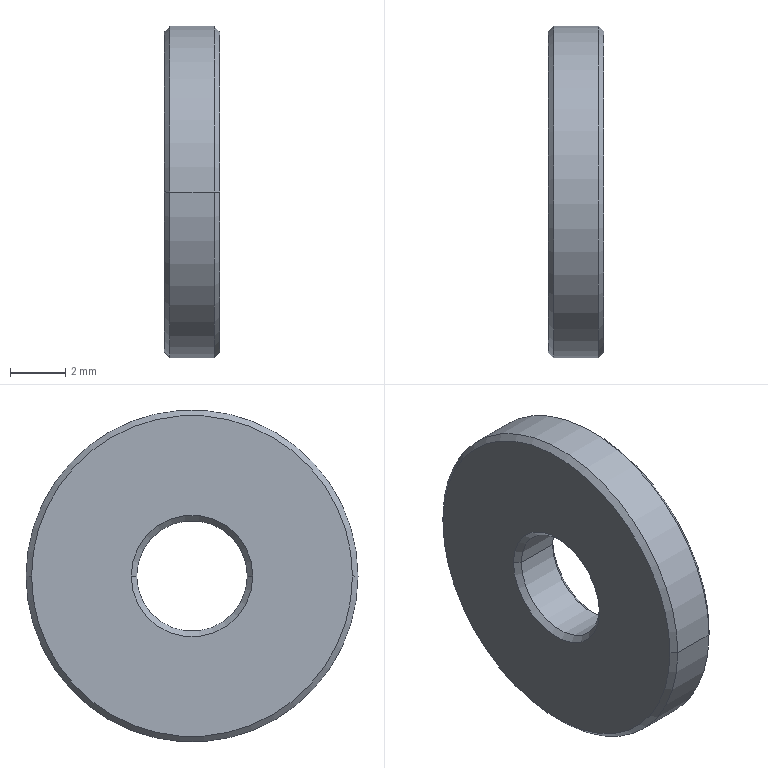Part | STEP file | wasmh12_4_2_2_03 | 1 solid | 14 faces | box 2 x 12 x 12 mm | volume 199.051 mm3 | cone 8 | cylinder 4 | plane 2 | commonest cylinder face diameters 4 x2 12 x2
STEP:
#1=CARTESIAN_POINT('',(0.,0.,0.));
#2=DIRECTION('',(0.,0.,1.));
#3=DIRECTION('',(1.,0.,0.));
#4=AXIS2_PLACEMENT_3D('',#1,#2,#3);
#5=CARTESIAN_POINT('',(0.2,-2.,0.));
#6=VERTEX_POINT('',#5);
#7=CARTESIAN_POINT('',(0.,-2.2,0.));
#8=VERTEX_POINT('',#7);
#9=CARTESIAN_POINT('',(0.,-2.2,0.));
#10=DIRECTION('',(-0.7071,-0.7071,0.));
#11=VECTOR('',#10,1.);
#12=LINE('',#9,#11);
#13=CARTESIAN_POINT('',(0.,0.,0.));
#14=DIRECTION('',(-1.,0.,0.));
#15=DIRECTION('',(0.,-1.,0.));
#16=AXIS2_PLACEMENT_3D('',#13,#14,#15);
#17=CONICAL_SURFACE('',#16,2.2,0.7854);
#18=CARTESIAN_POINT('',(6.283,0.));
#19=DIRECTION('',(0.,1.));
#20=VECTOR('',#19,1.);
#21=LINE('',#18,#20);
#22=(GEOMETRIC_REPRESENTATION_CONTEXT(2)PARAMETRIC_REPRESENTATION_CONTEXT()REPRESENTATION_CONTEXT('',''));
#23=DEFINITIONAL_REPRESENTATION('',(#21),#22);
#24=PCURVE('',#17,#23);
#25=CARTESIAN_POINT('',(0.,0.,0.));
#26=DIRECTION('',(-1.,0.,0.));
#27=DIRECTION('',(0.,-1.,0.));
#28=AXIS2_PLACEMENT_3D('',#25,#26,#27);
#29=CONICAL_SURFACE('',#28,2.2,0.7854);
#30=CARTESIAN_POINT('',(0.,0.));
#31=DIRECTION('',(0.,1.));
#32=VECTOR('',#31,1.);
#33=LINE('',#30,#32);
#34=(GEOMETRIC_REPRESENTATION_CONTEXT(2)PARAMETRIC_REPRESENTATION_CONTEXT()REPRESENTATION_CONTEXT('',''));
#35=DEFINITIONAL_REPRESENTATION('',(#33),#34);
#36=PCURVE('',#29,#35);
#37=SURFACE_CURVE('',#12,(#24,#36),.PCURVE_S1.);
#38=EDGE_CURVE('',#6,#8,#37,.T.);
#39=ORIENTED_EDGE('',*,*,#38,.T.);
#40=CARTESIAN_POINT('',(0.,2.2,0.));
#41=VERTEX_POINT('',#40);
#42=CARTESIAN_POINT('',(0.,0.,0.));
#43=DIRECTION('',(1.,0.,0.));
#44=DIRECTION('',(0.,-1.,0.));
#45=AXIS2_PLACEMENT_3D('',#42,#43,#44);
#46=CIRCLE('',#45,2.2);
#47=CARTESIAN_POINT('',(6.283,0.));
#48=DIRECTION('',(-1.,0.));
#49=VECTOR('',#48,1.);
#50=LINE('',#47,#49);
#51=(GEOMETRIC_REPRESENTATION_CONTEXT(2)PARAMETRIC_REPRESENTATION_CONTEXT()REPRESENTATION_CONTEXT('',''));
#52=DEFINITIONAL_REPRESENTATION('',(#50),#51);
#53=PCURVE('',#17,#52);
#54=CARTESIAN_POINT('',(0.,-4.,0.));
#55=DIRECTION('',(-1.,0.,0.));
#56=DIRECTION('',(0.,-1.,0.));
#57=AXIS2_PLACEMENT_3D('',#54,#55,#56);
#58=PLANE('',#57);
#59=CARTESIAN_POINT('',(-1.8,0.));
#60=CARTESIAN_POINT('',(-1.8,-3.811));
#61=CARTESIAN_POINT('',(-5.1,-1.905));
#62=CARTESIAN_POINT('',(-8.4,0.));
#63=CARTESIAN_POINT('',(-5.1,1.905));
#64=CARTESIAN_POINT('',(-1.8,3.811));
#65=CARTESIAN_POINT('',(-1.8,0.));
#66=(BOUNDED_CURVE()B_SPLINE_CURVE(2,(#59,#60,#61,#62,#63,#64,#65),.UNSPECIFIED.,.T.,.F.)B_SPLINE_CURVE_WITH_KNOTS((1,2,2,2,2,1),(-2.094,0.,2.094,4.189,6.283,8.378),.UNSPECIFIED.)CURVE()GEOMETRIC_REPRESENTATION_ITEM()RATIONAL_B_SPLINE_CURVE((1.,0.5,1.,0.5,1.,0.5,1.))REPRESENTATION_ITEM(''));
#67=(GEOMETRIC_REPRESENTATION_CONTEXT(2)PARAMETRIC_REPRESENTATION_CONTEXT()REPRESENTATION_CONTEXT('',''));
#68=DEFINITIONAL_REPRESENTATION('',(#66),#67);
#69=PCURVE('',#58,#68);
#70=SURFACE_CURVE('',#46,(#53,#69),.PCURVE_S1.);
#71=EDGE_CURVE('',#8,#41,#70,.T.);
#72=ORIENTED_EDGE('',*,*,#71,.T.);
#73=CARTESIAN_POINT('',(0.2,2.,0.));
#74=VERTEX_POINT('',#73);
#75=CARTESIAN_POINT('',(0.,2.2,0.));
#76=DIRECTION('',(-0.7071,0.7071,0.));
#77=VECTOR('',#76,1.);
#78=LINE('',#75,#77);
#79=CARTESIAN_POINT('',(3.142,0.));
#80=DIRECTION('',(0.,1.));
#81=VECTOR('',#80,1.);
#82=LINE('',#79,#81);
#83=(GEOMETRIC_REPRESENTATION_CONTEXT(2)PARAMETRIC_REPRESENTATION_CONTEXT()REPRESENTATION_CONTEXT('',''));
#84=DEFINITIONAL_REPRESENTATION('',(#82),#83);
#85=PCURVE('',#17,#84);
#86=CARTESIAN_POINT('',(3.142,0.));
#87=DIRECTION('',(0.,1.));
#88=VECTOR('',#87,1.);
#89=LINE('',#86,#88);
#90=(GEOMETRIC_REPRESENTATION_CONTEXT(2)PARAMETRIC_REPRESENTATION_CONTEXT()REPRESENTATION_CONTEXT('',''));
#91=DEFINITIONAL_REPRESENTATION('',(#89),#90);
#92=PCURVE('',#29,#91);
#93=SURFACE_CURVE('',#78,(#85,#92),.PCURVE_S1.);
#94=EDGE_CURVE('',#74,#41,#93,.T.);
#95=ORIENTED_EDGE('',*,*,#94,.F.);
#96=CARTESIAN_POINT('',(0.2,0.,0.));
#97=DIRECTION('',(-1.,0.,0.));
#98=DIRECTION('',(0.,-1.,0.));
#99=AXIS2_PLACEMENT_3D('',#96,#97,#98);
#100=CIRCLE('',#99,2.);
#101=CARTESIAN_POINT('',(0.,-0.2));
#102=DIRECTION('',(1.,0.));
#103=VECTOR('',#102,1.);
#104=LINE('',#101,#103);
#105=(GEOMETRIC_REPRESENTATION_CONTEXT(2)PARAMETRIC_REPRESENTATION_CONTEXT()REPRESENTATION_CONTEXT('',''));
#106=DEFINITIONAL_REPRESENTATION('',(#104),#105);
#107=PCURVE('',#17,#106);
#108=CARTESIAN_POINT('',(1.,0.,0.));
#109=DIRECTION('',(-1.,0.,0.));
#110=DIRECTION('',(0.,-1.,0.));
#111=AXIS2_PLACEMENT_3D('',#108,#109,#110);
#112=CYLINDRICAL_SURFACE('',#111,2.);
#113=CARTESIAN_POINT('',(0.,0.8));
#114=DIRECTION('',(1.,0.));
#115=VECTOR('',#114,1.);
#116=LINE('',#113,#115);
#117=(GEOMETRIC_REPRESENTATION_CONTEXT(2)PARAMETRIC_REPRESENTATION_CONTEXT()REPRESENTATION_CONTEXT('',''));
#118=DEFINITIONAL_REPRESENTATION('',(#116),#117);
#119=PCURVE('',#112,#118);
#120=SURFACE_CURVE('',#100,(#107,#119),.PCURVE_S1.);
#121=EDGE_CURVE('',#74,#6,#120,.T.);
#122=ORIENTED_EDGE('',*,*,#121,.T.);
#123=EDGE_LOOP('',(#39,#72,#95,#122));
#124=FACE_BOUND('',#123,.F.);
#125=ADVANCED_FACE('',(#124),#17,.F.);
#126=CARTESIAN_POINT('',(0.,-5.8,0.));
#127=VERTEX_POINT('',#126);
#128=CARTESIAN_POINT('',(0.,5.8,0.));
#129=VERTEX_POINT('',#128);
#130=CARTESIAN_POINT('',(0.,0.,0.));
#131=DIRECTION('',(-1.,0.,0.));
#132=DIRECTION('',(0.,1.,0.));
#133=AXIS2_PLACEMENT_3D('',#130,#131,#132);
#134=CIRCLE('',#133,5.8);
#135=CARTESIAN_POINT('',(0.2,0.,0.));
#136=DIRECTION('',(1.,0.,0.));
#137=DIRECTION('',(0.,1.,0.));
#138=AXIS2_PLACEMENT_3D('',#135,#136,#137);
#139=CONICAL_SURFACE('',#138,6.,0.7854);
#140=CARTESIAN_POINT('',(6.283,-0.2));
#141=DIRECTION('',(-1.,0.));
#142=VECTOR('',#141,1.);
#143=LINE('',#140,#142);
#144=(GEOMETRIC_REPRESENTATION_CONTEXT(2)PARAMETRIC_REPRESENTATION_CONTEXT()REPRESENTATION_CONTEXT('',''));
#145=DEFINITIONAL_REPRESENTATION('',(#143),#144);
#146=PCURVE('',#139,#145);
#147=CARTESIAN_POINT('',(-4.,0.));
#148=DIRECTION('',(-1.,0.));
#149=AXIS2_PLACEMENT_2D('',#147,#148);
#150=CIRCLE('',#149,5.8);
#151=(GEOMETRIC_REPRESENTATION_CONTEXT(2)PARAMETRIC_REPRESENTATION_CONTEXT()REPRESENTATION_CONTEXT('',''));
#152=DEFINITIONAL_REPRESENTATION('',(#150),#151);
#153=PCURVE('',#58,#152);
#154=SURFACE_CURVE('',#134,(#146,#153),.PCURVE_S1.);
#155=EDGE_CURVE('',#127,#129,#154,.T.);
#156=ORIENTED_EDGE('',*,*,#155,.F.);
#157=CARTESIAN_POINT('',(0.2,-6.,0.));
#158=VERTEX_POINT('',#157);
#159=CARTESIAN_POINT('',(0.2,-6.,0.));
#160=DIRECTION('',(0.7071,-0.7071,0.));
#161=VECTOR('',#160,1.);
#162=LINE('',#159,#161);
#163=CARTESIAN_POINT('',(3.142,0.));
#164=DIRECTION('',(0.,1.));
#165=VECTOR('',#164,1.);
#166=LINE('',#163,#165);
#167=(GEOMETRIC_REPRESENTATION_CONTEXT(2)PARAMETRIC_REPRESENTATION_CONTEXT()REPRESENTATION_CONTEXT('',''));
#168=DEFINITIONAL_REPRESENTATION('',(#166),#167);
#169=PCURVE('',#139,#168);
#170=CARTESIAN_POINT('',(0.2,0.,0.));
#171=DIRECTION('',(1.,0.,0.));
#172=DIRECTION('',(0.,1.,0.));
#173=AXIS2_PLACEMENT_3D('',#170,#171,#172);
#174=CONICAL_SURFACE('',#173,6.,0.7854);
#175=CARTESIAN_POINT('',(3.142,0.));
#176=DIRECTION('',(0.,1.));
#177=VECTOR('',#176,1.);
#178=LINE('',#175,#177);
#179=(GEOMETRIC_REPRESENTATION_CONTEXT(2)PARAMETRIC_REPRESENTATION_CONTEXT()REPRESENTATION_CONTEXT('',''));
#180=DEFINITIONAL_REPRESENTATION('',(#178),#179);
#181=PCURVE('',#174,#180);
#182=SURFACE_CURVE('',#162,(#169,#181),.PCURVE_S1.);
#183=EDGE_CURVE('',#127,#158,#182,.T.);
#184=ORIENTED_EDGE('',*,*,#183,.T.);
#185=CARTESIAN_POINT('',(0.2,6.,0.));
#186=VERTEX_POINT('',#185);
#187=CARTESIAN_POINT('',(0.2,0.,0.));
#188=DIRECTION('',(-1.,0.,0.));
#189=DIRECTION('',(0.,-1.,0.));
#190=AXIS2_PLACEMENT_3D('',#187,#188,#189);
#191=CIRCLE('',#190,6.);
#192=CARTESIAN_POINT('',(3.142,0.));
#193=DIRECTION('',(-1.,0.));
#194=VECTOR('',#193,1.);
#195=LINE('',#192,#194);
#196=(GEOMETRIC_REPRESENTATION_CONTEXT(2)PARAMETRIC_REPRESENTATION_CONTEXT()REPRESENTATION_CONTEXT('',''));
#197=DEFINITIONAL_REPRESENTATION('',(#195),#196);
#198=PCURVE('',#139,#197);
#199=CARTESIAN_POINT('',(1.,0.,0.));
#200=DIRECTION('',(-1.,0.,0.));
#201=DIRECTION('',(0.,-1.,0.));
#202=AXIS2_PLACEMENT_3D('',#199,#200,#201);
#203=CYLINDRICAL_SURFACE('',#202,6.);
#204=CARTESIAN_POINT('',(0.,0.8));
#205=DIRECTION('',(1.,0.));
#206=VECTOR('',#205,1.);
#207=LINE('',#204,#206);
#208=(GEOMETRIC_REPRESENTATION_CONTEXT(2)PARAMETRIC_REPRESENTATION_CONTEXT()REPRESENTATION_CONTEXT('',''));
#209=DEFINITIONAL_REPRESENTATION('',(#207),#208);
#210=PCURVE('',#203,#209);
#211=SURFACE_CURVE('',#191,(#198,#210),.PCURVE_S1.);
#212=EDGE_CURVE('',#158,#186,#211,.T.);
#213=ORIENTED_EDGE('',*,*,#212,.T.);
#214=CARTESIAN_POINT('',(0.2,6.,0.));
#215=DIRECTION('',(0.7071,0.7071,0.));
#216=VECTOR('',#215,1.);
#217=LINE('',#214,#216);
#218=CARTESIAN_POINT('',(0.,0.));
#219=DIRECTION('',(0.,1.));
#220=VECTOR('',#219,1.);
#221=LINE('',#218,#220);
#222=(GEOMETRIC_REPRESENTATION_CONTEXT(2)PARAMETRIC_REPRESENTATION_CONTEXT()REPRESENTATION_CONTEXT('',''));
#223=DEFINITIONAL_REPRESENTATION('',(#221),#222);
#224=PCURVE('',#139,#223);
#225=CARTESIAN_POINT('',(6.283,0.));
#226=DIRECTION('',(0.,1.));
#227=VECTOR('',#226,1.);
#228=LINE('',#225,#227);
#229=(GEOMETRIC_REPRESENTATION_CONTEXT(2)PARAMETRIC_REPRESENTATION_CONTEXT()REPRESENTATION_CONTEXT('',''));
#230=DEFINITIONAL_REPRESENTATION('',(#228),#229);
#231=PCURVE('',#174,#230);
#232=SURFACE_CURVE('',#217,(#224,#231),.PCURVE_S1.);
#233=EDGE_CURVE('',#129,#186,#232,.T.);
#234=ORIENTED_EDGE('',*,*,#233,.F.);
#235=EDGE_LOOP('',(#156,#184,#213,#234));
#236=FACE_BOUND('',#235,.T.);
#237=ADVANCED_FACE('',(#236),#139,.T.);
#238=CARTESIAN_POINT('',(1.8,-2.,0.));
#239=VERTEX_POINT('',#238);
#240=CARTESIAN_POINT('',(1.,-2.,0.));
#241=DIRECTION('',(-1.,0.,0.));
#242=VECTOR('',#241,1.);
#243=LINE('',#240,#242);
#244=CARTESIAN_POINT('',(6.283,0.));
#245=DIRECTION('',(0.,1.));
#246=VECTOR('',#245,1.);
#247=LINE('',#244,#246);
#248=(GEOMETRIC_REPRESENTATION_CONTEXT(2)PARAMETRIC_REPRESENTATION_CONTEXT()REPRESENTATION_CONTEXT('',''));
#249=DEFINITIONAL_REPRESENTATION('',(#247),#248);
#250=PCURVE('',#112,#249);
#251=CARTESIAN_POINT('',(1.,0.,0.));
#252=DIRECTION('',(-1.,0.,0.));
#253=DIRECTION('',(0.,-1.,0.));
#254=AXIS2_PLACEMENT_3D('',#251,#252,#253);
#255=CYLINDRICAL_SURFACE('',#254,2.);
#256=CARTESIAN_POINT('',(0.,0.));
#257=DIRECTION('',(0.,1.));
#258=VECTOR('',#257,1.);
#259=LINE('',#256,#258);
#260=(GEOMETRIC_REPRESENTATION_CONTEXT(2)PARAMETRIC_REPRESENTATION_CONTEXT()REPRESENTATION_CONTEXT('',''));
#261=DEFINITIONAL_REPRESENTATION('',(#259),#260);
#262=PCURVE('',#255,#261);
#263=SURFACE_CURVE('',#243,(#250,#262),.PCURVE_S1.);
#264=EDGE_CURVE('',#239,#6,#263,.T.);
#265=ORIENTED_EDGE('',*,*,#264,.T.);
#266=ORIENTED_EDGE('',*,*,#121,.F.);
#267=CARTESIAN_POINT('',(1.8,2.,0.));
#268=VERTEX_POINT('',#267);
#269=CARTESIAN_POINT('',(1.,2.,0.));
#270=DIRECTION('',(-1.,0.,0.));
#271=VECTOR('',#270,1.);
#272=LINE('',#269,#271);
#273=CARTESIAN_POINT('',(3.142,0.));
#274=DIRECTION('',(0.,1.));
#275=VECTOR('',#274,1.);
#276=LINE('',#273,#275);
#277=(GEOMETRIC_REPRESENTATION_CONTEXT(2)PARAMETRIC_REPRESENTATION_CONTEXT()REPRESENTATION_CONTEXT('',''));
#278=DEFINITIONAL_REPRESENTATION('',(#276),#277);
#279=PCURVE('',#112,#278);
#280=CARTESIAN_POINT('',(3.142,0.));
#281=DIRECTION('',(0.,1.));
#282=VECTOR('',#281,1.);
#283=LINE('',#280,#282);
#284=(GEOMETRIC_REPRESENTATION_CONTEXT(2)PARAMETRIC_REPRESENTATION_CONTEXT()REPRESENTATION_CONTEXT('',''));
#285=DEFINITIONAL_REPRESENTATION('',(#283),#284);
#286=PCURVE('',#255,#285);
#287=SURFACE_CURVE('',#272,(#279,#286),.PCURVE_S1.);
#288=EDGE_CURVE('',#268,#74,#287,.T.);
#289=ORIENTED_EDGE('',*,*,#288,.F.);
#290=CARTESIAN_POINT('',(1.8,0.,0.));
#291=DIRECTION('',(-1.,0.,0.));
#292=DIRECTION('',(0.,-1.,0.));
#293=AXIS2_PLACEMENT_3D('',#290,#291,#292);
#294=CIRCLE('',#293,2.);
#295=CARTESIAN_POINT('',(0.,-0.8));
#296=DIRECTION('',(1.,0.));
#297=VECTOR('',#296,1.);
#298=LINE('',#295,#297);
#299=(GEOMETRIC_REPRESENTATION_CONTEXT(2)PARAMETRIC_REPRESENTATION_CONTEXT()REPRESENTATION_CONTEXT('',''));
#300=DEFINITIONAL_REPRESENTATION('',(#298),#299);
#301=PCURVE('',#112,#300);
#302=CARTESIAN_POINT('',(2.,0.,0.));
#303=DIRECTION('',(1.,0.,0.));
#304=DIRECTION('',(0.,1.,0.));
#305=AXIS2_PLACEMENT_3D('',#302,#303,#304);
#306=CONICAL_SURFACE('',#305,2.2,0.7854);
#307=CARTESIAN_POINT('',(9.425,-0.2));
#308=DIRECTION('',(-1.,0.));
#309=VECTOR('',#308,1.);
#310=LINE('',#307,#309);
#311=(GEOMETRIC_REPRESENTATION_CONTEXT(2)PARAMETRIC_REPRESENTATION_CONTEXT()REPRESENTATION_CONTEXT('',''));
#312=DEFINITIONAL_REPRESENTATION('',(#310),#311);
#313=PCURVE('',#306,#312);
#314=SURFACE_CURVE('',#294,(#301,#313),.PCURVE_S1.);
#315=EDGE_CURVE('',#268,#239,#314,.T.);
#316=ORIENTED_EDGE('',*,*,#315,.T.);
#317=EDGE_LOOP('',(#265,#266,#289,#316));
#318=FACE_BOUND('',#317,.F.);
#319=ADVANCED_FACE('',(#318),#112,.F.);
#320=CARTESIAN_POINT('',(1.8,-6.,0.));
#321=VERTEX_POINT('',#320);
#322=CARTESIAN_POINT('',(1.8,6.,0.));
#323=VERTEX_POINT('',#322);
#324=CARTESIAN_POINT('',(1.8,0.,0.));
#325=DIRECTION('',(-1.,0.,0.));
#326=DIRECTION('',(0.,-1.,0.));
#327=AXIS2_PLACEMENT_3D('',#324,#325,#326);
#328=CIRCLE('',#327,6.);
#329=CARTESIAN_POINT('',(0.,-0.8));
#330=DIRECTION('',(1.,0.));
#331=VECTOR('',#330,1.);
#332=LINE('',#329,#331);
#333=(GEOMETRIC_REPRESENTATION_CONTEXT(2)PARAMETRIC_REPRESENTATION_CONTEXT()REPRESENTATION_CONTEXT('',''));
#334=DEFINITIONAL_REPRESENTATION('',(#332),#333);
#335=PCURVE('',#203,#334);
#336=CARTESIAN_POINT('',(1.8,0.,0.));
#337=DIRECTION('',(-1.,0.,0.));
#338=DIRECTION('',(0.,-1.,0.));
#339=AXIS2_PLACEMENT_3D('',#336,#337,#338);
#340=CONICAL_SURFACE('',#339,6.,0.7854);
#341=CARTESIAN_POINT('',(0.,0.));
#342=DIRECTION('',(1.,0.));
#343=VECTOR('',#342,1.);
#344=LINE('',#341,#343);
#345=(GEOMETRIC_REPRESENTATION_CONTEXT(2)PARAMETRIC_REPRESENTATION_CONTEXT()REPRESENTATION_CONTEXT('',''));
#346=DEFINITIONAL_REPRESENTATION('',(#344),#345);
#347=PCURVE('',#340,#346);
#348=SURFACE_CURVE('',#328,(#335,#347),.PCURVE_S1.);
#349=EDGE_CURVE('',#321,#323,#348,.T.);
#350=ORIENTED_EDGE('',*,*,#349,.T.);
#351=CARTESIAN_POINT('',(1.,6.,0.));
#352=DIRECTION('',(-1.,0.,0.));
#353=VECTOR('',#352,1.);
#354=LINE('',#351,#353);
#355=CARTESIAN_POINT('',(3.142,0.));
#356=DIRECTION('',(0.,1.));
#357=VECTOR('',#356,1.);
#358=LINE('',#355,#357);
#359=(GEOMETRIC_REPRESENTATION_CONTEXT(2)PARAMETRIC_REPRESENTATION_CONTEXT()REPRESENTATION_CONTEXT('',''));
#360=DEFINITIONAL_REPRESENTATION('',(#358),#359);
#361=PCURVE('',#203,#360);
#362=CARTESIAN_POINT('',(1.,0.,0.));
#363=DIRECTION('',(-1.,0.,0.));
#364=DIRECTION('',(0.,-1.,0.));
#365=AXIS2_PLACEMENT_3D('',#362,#363,#364);
#366=CYLINDRICAL_SURFACE('',#365,6.);
#367=CARTESIAN_POINT('',(3.142,0.));
#368=DIRECTION('',(0.,1.));
#369=VECTOR('',#368,1.);
#370=LINE('',#367,#369);
#371=(GEOMETRIC_REPRESENTATION_CONTEXT(2)PARAMETRIC_REPRESENTATION_CONTEXT()REPRESENTATION_CONTEXT('',''));
#372=DEFINITIONAL_REPRESENTATION('',(#370),#371);
#373=PCURVE('',#366,#372);
#374=SURFACE_CURVE('',#354,(#361,#373),.PCURVE_S1.);
#375=EDGE_CURVE('',#323,#186,#374,.T.);
#376=ORIENTED_EDGE('',*,*,#375,.T.);
#377=ORIENTED_EDGE('',*,*,#212,.F.);
#378=CARTESIAN_POINT('',(1.,-6.,0.));
#379=DIRECTION('',(-1.,0.,0.));
#380=VECTOR('',#379,1.);
#381=LINE('',#378,#380);
#382=CARTESIAN_POINT('',(0.,0.));
#383=DIRECTION('',(0.,1.));
#384=VECTOR('',#383,1.);
#385=LINE('',#382,#384);
#386=(GEOMETRIC_REPRESENTATION_CONTEXT(2)PARAMETRIC_REPRESENTATION_CONTEXT()REPRESENTATION_CONTEXT('',''));
#387=DEFINITIONAL_REPRESENTATION('',(#385),#386);
#388=PCURVE('',#203,#387);
#389=CARTESIAN_POINT('',(6.283,0.));
#390=DIRECTION('',(0.,1.));
#391=VECTOR('',#390,1.);
#392=LINE('',#389,#391);
#393=(GEOMETRIC_REPRESENTATION_CONTEXT(2)PARAMETRIC_REPRESENTATION_CONTEXT()REPRESENTATION_CONTEXT('',''));
#394=DEFINITIONAL_REPRESENTATION('',(#392),#393);
#395=PCURVE('',#366,#394);
#396=SURFACE_CURVE('',#381,(#388,#395),.PCURVE_S1.);
#397=EDGE_CURVE('',#321,#158,#396,.T.);
#398=ORIENTED_EDGE('',*,*,#397,.F.);
#399=EDGE_LOOP('',(#350,#376,#377,#398));
#400=FACE_BOUND('',#399,.T.);
#401=ADVANCED_FACE('',(#400),#203,.T.);
#402=CARTESIAN_POINT('',(2.,2.2,0.));
#403=VERTEX_POINT('',#402);
#404=CARTESIAN_POINT('',(2.,2.2,0.));
#405=DIRECTION('',(0.7071,0.7071,0.));
#406=VECTOR('',#405,1.);
#407=LINE('',#404,#406);
#408=CARTESIAN_POINT('',(6.283,0.));
#409=DIRECTION('',(0.,1.));
#410=VECTOR('',#409,1.);
#411=LINE('',#408,#410);
#412=(GEOMETRIC_REPRESENTATION_CONTEXT(2)PARAMETRIC_REPRESENTATION_CONTEXT()REPRESENTATION_CONTEXT('',''));
#413=DEFINITIONAL_REPRESENTATION('',(#411),#412);
#414=PCURVE('',#306,#413);
#415=CARTESIAN_POINT('',(2.,0.,0.));
#416=DIRECTION('',(1.,0.,0.));
#417=DIRECTION('',(0.,1.,0.));
#418=AXIS2_PLACEMENT_3D('',#415,#416,#417);
#419=CONICAL_SURFACE('',#418,2.2,0.7854);
#420=CARTESIAN_POINT('',(0.,0.));
#421=DIRECTION('',(0.,1.));
#422=VECTOR('',#421,1.);
#423=LINE('',#420,#422);
#424=(GEOMETRIC_REPRESENTATION_CONTEXT(2)PARAMETRIC_REPRESENTATION_CONTEXT()REPRESENTATION_CONTEXT('',''));
#425=DEFINITIONAL_REPRESENTATION('',(#423),#424);
#426=PCURVE('',#419,#425);
#427=SURFACE_CURVE('',#407,(#414,#426),.PCURVE_S1.);
#428=EDGE_CURVE('',#268,#403,#427,.T.);
#429=ORIENTED_EDGE('',*,*,#428,.T.);
#430=CARTESIAN_POINT('',(2.,-2.2,0.));
#431=VERTEX_POINT('',#430);
#432=CARTESIAN_POINT('',(2.,0.,0.));
#433=DIRECTION('',(-1.,0.,0.));
#434=DIRECTION('',(0.,1.,0.));
#435=AXIS2_PLACEMENT_3D('',#432,#433,#434);
#436=CIRCLE('',#435,2.2);
#437=CARTESIAN_POINT('',(6.283,0.));
#438=DIRECTION('',(-1.,0.));
#439=VECTOR('',#438,1.);
#440=LINE('',#437,#439);
#441=(GEOMETRIC_REPRESENTATION_CONTEXT(2)PARAMETRIC_REPRESENTATION_CONTEXT()REPRESENTATION_CONTEXT('',''));
#442=DEFINITIONAL_REPRESENTATION('',(#440),#441);
#443=PCURVE('',#306,#442);
#444=CARTESIAN_POINT('',(2.,-4.,0.));
#445=DIRECTION('',(1.,0.,0.));
#446=DIRECTION('',(0.,1.,0.));
#447=AXIS2_PLACEMENT_3D('',#444,#445,#446);
#448=PLANE('',#447);
#449=CARTESIAN_POINT('',(6.2,0.));
#450=CARTESIAN_POINT('',(6.2,-3.811));
#451=CARTESIAN_POINT('',(2.9,-1.905));
#452=CARTESIAN_POINT('',(-0.4,0.));
#453=CARTESIAN_POINT('',(2.9,1.905));
#454=CARTESIAN_POINT('',(6.2,3.811));
#455=CARTESIAN_POINT('',(6.2,0.));
#456=(BOUNDED_CURVE()B_SPLINE_CURVE(2,(#449,#450,#451,#452,#453,#454,#455),.UNSPECIFIED.,.T.,.F.)B_SPLINE_CURVE_WITH_KNOTS((1,2,2,2,2,1),(-2.094,0.,2.094,4.189,6.283,8.378),.UNSPECIFIED.)CURVE()GEOMETRIC_REPRESENTATION_ITEM()RATIONAL_B_SPLINE_CURVE((1.,0.5,1.,0.5,1.,0.5,1.))REPRESENTATION_ITEM(''));
#457=(GEOMETRIC_REPRESENTATION_CONTEXT(2)PARAMETRIC_REPRESENTATION_CONTEXT()REPRESENTATION_CONTEXT('',''));
#458=DEFINITIONAL_REPRESENTATION('',(#456),#457);
#459=PCURVE('',#448,#458);
#460=SURFACE_CURVE('',#436,(#443,#459),.PCURVE_S1.);
#461=EDGE_CURVE('',#403,#431,#460,.T.);
#462=ORIENTED_EDGE('',*,*,#461,.T.);
#463=CARTESIAN_POINT('',(2.,-2.2,0.));
#464=DIRECTION('',(0.7071,-0.7071,0.));
#465=VECTOR('',#464,1.);
#466=LINE('',#463,#465);
#467=CARTESIAN_POINT('',(3.142,0.));
#468=DIRECTION('',(0.,1.));
#469=VECTOR('',#468,1.);
#470=LINE('',#467,#469);
#471=(GEOMETRIC_REPRESENTATION_CONTEXT(2)PARAMETRIC_REPRESENTATION_CONTEXT()REPRESENTATION_CONTEXT('',''));
#472=DEFINITIONAL_REPRESENTATION('',(#470),#471);
#473=PCURVE('',#306,#472);
#474=CARTESIAN_POINT('',(3.142,0.));
#475=DIRECTION('',(0.,1.));
#476=VECTOR('',#475,1.);
#477=LINE('',#474,#476);
#478=(GEOMETRIC_REPRESENTATION_CONTEXT(2)PARAMETRIC_REPRESENTATION_CONTEXT()REPRESENTATION_CONTEXT('',''));
#479=DEFINITIONAL_REPRESENTATION('',(#477),#478);
#480=PCURVE('',#419,#479);
#481=SURFACE_CURVE('',#466,(#473,#480),.PCURVE_S1.);
#482=EDGE_CURVE('',#239,#431,#481,.T.);
#483=ORIENTED_EDGE('',*,*,#482,.F.);
#484=ORIENTED_EDGE('',*,*,#315,.F.);
#485=EDGE_LOOP('',(#429,#462,#483,#484));
#486=FACE_BOUND('',#485,.F.);
#487=ADVANCED_FACE('',(#486),#306,.F.);
#488=CARTESIAN_POINT('',(2.,-5.8,0.));
#489=VERTEX_POINT('',#488);
#490=CARTESIAN_POINT('',(2.,5.8,0.));
#491=VERTEX_POINT('',#490);
#492=CARTESIAN_POINT('',(2.,0.,0.));
#493=DIRECTION('',(-1.,0.,0.));
#494=DIRECTION('',(0.,-1.,0.));
#495=AXIS2_PLACEMENT_3D('',#492,#493,#494);
#496=CIRCLE('',#495,5.8);
#497=CARTESIAN_POINT('',(0.,-0.2));
#498=DIRECTION('',(1.,0.));
#499=VECTOR('',#498,1.);
#500=LINE('',#497,#499);
#501=(GEOMETRIC_REPRESENTATION_CONTEXT(2)PARAMETRIC_REPRESENTATION_CONTEXT()REPRESENTATION_CONTEXT('',''));
#502=DEFINITIONAL_REPRESENTATION('',(#500),#501);
#503=PCURVE('',#340,#502);
#504=CARTESIAN_POINT('',(-1.8,0.));
#505=CARTESIAN_POINT('',(-1.8,10.046));
#506=CARTESIAN_POINT('',(6.9,5.023));
#507=CARTESIAN_POINT('',(15.6,0.));
#508=CARTESIAN_POINT('',(6.9,-5.023));
#509=CARTESIAN_POINT('',(-1.8,-10.046));
#510=CARTESIAN_POINT('',(-1.8,0.));
#511=(BOUNDED_CURVE()B_SPLINE_CURVE(2,(#504,#505,#506,#507,#508,#509,#510),.UNSPECIFIED.,.T.,.F.)B_SPLINE_CURVE_WITH_KNOTS((1,2,2,2,2,1),(-2.094,0.,2.094,4.189,6.283,8.378),.UNSPECIFIED.)CURVE()GEOMETRIC_REPRESENTATION_ITEM()RATIONAL_B_SPLINE_CURVE((1.,0.5,1.,0.5,1.,0.5,1.))REPRESENTATION_ITEM(''));
#512=(GEOMETRIC_REPRESENTATION_CONTEXT(2)PARAMETRIC_REPRESENTATION_CONTEXT()REPRESENTATION_CONTEXT('',''));
#513=DEFINITIONAL_REPRESENTATION('',(#511),#512);
#514=PCURVE('',#448,#513);
#515=SURFACE_CURVE('',#496,(#503,#514),.PCURVE_S1.);
#516=EDGE_CURVE('',#489,#491,#515,.T.);
#517=ORIENTED_EDGE('',*,*,#516,.T.);
#518=CARTESIAN_POINT('',(1.8,6.,0.));
#519=DIRECTION('',(-0.7071,0.7071,0.));
#520=VECTOR('',#519,1.);
#521=LINE('',#518,#520);
#522=CARTESIAN_POINT('',(3.142,0.));
#523=DIRECTION('',(0.,1.));
#524=VECTOR('',#523,1.);
#525=LINE('',#522,#524);
#526=(GEOMETRIC_REPRESENTATION_CONTEXT(2)PARAMETRIC_REPRESENTATION_CONTEXT()REPRESENTATION_CONTEXT('',''));
#527=DEFINITIONAL_REPRESENTATION('',(#525),#526);
#528=PCURVE('',#340,#527);
#529=CARTESIAN_POINT('',(1.8,0.,0.));
#530=DIRECTION('',(-1.,0.,0.));
#531=DIRECTION('',(0.,-1.,0.));
#532=AXIS2_PLACEMENT_3D('',#529,#530,#531);
#533=CONICAL_SURFACE('',#532,6.,0.7854);
#534=CARTESIAN_POINT('',(3.142,0.));
#535=DIRECTION('',(0.,1.));
#536=VECTOR('',#535,1.);
#537=LINE('',#534,#536);
#538=(GEOMETRIC_REPRESENTATION_CONTEXT(2)PARAMETRIC_REPRESENTATION_CONTEXT()REPRESENTATION_CONTEXT('',''));
#539=DEFINITIONAL_REPRESENTATION('',(#537),#538);
#540=PCURVE('',#533,#539);
#541=SURFACE_CURVE('',#521,(#528,#540),.PCURVE_S1.);
#542=EDGE_CURVE('',#491,#323,#541,.T.);
#543=ORIENTED_EDGE('',*,*,#542,.T.);
#544=ORIENTED_EDGE('',*,*,#349,.F.);
#545=CARTESIAN_POINT('',(1.8,-6.,0.));
#546=DIRECTION('',(-0.7071,-0.7071,0.));
#547=VECTOR('',#546,1.);
#548=LINE('',#545,#547);
#549=CARTESIAN_POINT('',(0.,0.));
#550=DIRECTION('',(0.,1.));
#551=VECTOR('',#550,1.);
#552=LINE('',#549,#551);
#553=(GEOMETRIC_REPRESENTATION_CONTEXT(2)PARAMETRIC_REPRESENTATION_CONTEXT()REPRESENTATION_CONTEXT('',''));
#554=DEFINITIONAL_REPRESENTATION('',(#552),#553);
#555=PCURVE('',#340,#554);
#556=CARTESIAN_POINT('',(6.283,0.));
#557=DIRECTION('',(0.,1.));
#558=VECTOR('',#557,1.);
#559=LINE('',#556,#558);
#560=(GEOMETRIC_REPRESENTATION_CONTEXT(2)PARAMETRIC_REPRESENTATION_CONTEXT()REPRESENTATION_CONTEXT('',''));
#561=DEFINITIONAL_REPRESENTATION('',(#559),#560);
#562=PCURVE('',#533,#561);
#563=SURFACE_CURVE('',#548,(#555,#562),.PCURVE_S1.);
#564=EDGE_CURVE('',#489,#321,#563,.T.);
#565=ORIENTED_EDGE('',*,*,#564,.F.);
#566=EDGE_LOOP('',(#517,#543,#544,#565));
#567=FACE_BOUND('',#566,.T.);
#568=ADVANCED_FACE('',(#567),#340,.T.);
#569=ORIENTED_EDGE('',*,*,#71,.T.);
#570=CARTESIAN_POINT('',(0.,0.,0.));
#571=DIRECTION('',(1.,0.,0.));
#572=DIRECTION('',(0.,-1.,0.));
#573=AXIS2_PLACEMENT_3D('',#570,#571,#572);
#574=CIRCLE('',#573,2.2);
#575=CARTESIAN_POINT('',(-1.8,0.));
#576=CARTESIAN_POINT('',(-1.8,-3.811));
#577=CARTESIAN_POINT('',(-5.1,-1.905));
#578=CARTESIAN_POINT('',(-8.4,0.));
#579=CARTESIAN_POINT('',(-5.1,1.905));
#580=CARTESIAN_POINT('',(-1.8,3.811));
#581=CARTESIAN_POINT('',(-1.8,0.));
#582=(BOUNDED_CURVE()B_SPLINE_CURVE(2,(#575,#576,#577,#578,#579,#580,#581),.UNSPECIFIED.,.T.,.F.)B_SPLINE_CURVE_WITH_KNOTS((1,2,2,2,2,1),(-2.094,0.,2.094,4.189,6.283,8.378),.UNSPECIFIED.)CURVE()GEOMETRIC_REPRESENTATION_ITEM()RATIONAL_B_SPLINE_CURVE((1.,0.5,1.,0.5,1.,0.5,1.))REPRESENTATION_ITEM(''));
#583=(GEOMETRIC_REPRESENTATION_CONTEXT(2)PARAMETRIC_REPRESENTATION_CONTEXT()REPRESENTATION_CONTEXT('',''));
#584=DEFINITIONAL_REPRESENTATION('',(#582),#583);
#585=PCURVE('',#58,#584);
#586=CARTESIAN_POINT('',(6.283,0.));
#587=DIRECTION('',(-1.,0.));
#588=VECTOR('',#587,1.);
#589=LINE('',#586,#588);
#590=(GEOMETRIC_REPRESENTATION_CONTEXT(2)PARAMETRIC_REPRESENTATION_CONTEXT()REPRESENTATION_CONTEXT('',''));
#591=DEFINITIONAL_REPRESENTATION('',(#589),#590);
#592=PCURVE('',#29,#591);
#593=SURFACE_CURVE('',#574,(#585,#592),.PCURVE_S1.);
#594=EDGE_CURVE('',#41,#8,#593,.T.);
#595=ORIENTED_EDGE('',*,*,#594,.T.);
#596=EDGE_LOOP('',(#569,#595));
#597=FACE_BOUND('',#596,.T.);
#598=CARTESIAN_POINT('',(0.,0.,0.));
#599=DIRECTION('',(-1.,0.,0.));
#600=DIRECTION('',(0.,1.,0.));
#601=AXIS2_PLACEMENT_3D('',#598,#599,#600);
#602=CIRCLE('',#601,5.8);
#603=CARTESIAN_POINT('',(-4.,0.));
#604=DIRECTION('',(-1.,0.));
#605=AXIS2_PLACEMENT_2D('',#603,#604);
#606=CIRCLE('',#605,5.8);
#607=(GEOMETRIC_REPRESENTATION_CONTEXT(2)PARAMETRIC_REPRESENTATION_CONTEXT()REPRESENTATION_CONTEXT('',''));
#608=DEFINITIONAL_REPRESENTATION('',(#606),#607);
#609=PCURVE('',#58,#608);
#610=CARTESIAN_POINT('',(6.283,-0.2));
#611=DIRECTION('',(-1.,0.));
#612=VECTOR('',#611,1.);
#613=LINE('',#610,#612);
#614=(GEOMETRIC_REPRESENTATION_CONTEXT(2)PARAMETRIC_REPRESENTATION_CONTEXT()REPRESENTATION_CONTEXT('',''));
#615=DEFINITIONAL_REPRESENTATION('',(#613),#614);
#616=PCURVE('',#174,#615);
#617=SURFACE_CURVE('',#602,(#609,#616),.PCURVE_S1.);
#618=EDGE_CURVE('',#129,#127,#617,.T.);
#619=ORIENTED_EDGE('',*,*,#618,.T.);
#620=ORIENTED_EDGE('',*,*,#155,.T.);
#621=EDGE_LOOP('',(#619,#620));
#622=FACE_BOUND('',#621,.T.);
#623=ADVANCED_FACE('',(#597,#622),#58,.T.);
#624=ORIENTED_EDGE('',*,*,#594,.T.);
#625=ORIENTED_EDGE('',*,*,#38,.F.);
#626=CARTESIAN_POINT('',(0.2,0.,0.));
#627=DIRECTION('',(-1.,0.,0.));
#628=DIRECTION('',(0.,-1.,0.));
#629=AXIS2_PLACEMENT_3D('',#626,#627,#628);
#630=CIRCLE('',#629,2.);
#631=CARTESIAN_POINT('',(0.,-0.2));
#632=DIRECTION('',(1.,0.));
#633=VECTOR('',#632,1.);
#634=LINE('',#631,#633);
#635=(GEOMETRIC_REPRESENTATION_CONTEXT(2)PARAMETRIC_REPRESENTATION_CONTEXT()REPRESENTATION_CONTEXT('',''));
#636=DEFINITIONAL_REPRESENTATION('',(#634),#635);
#637=PCURVE('',#29,#636);
#638=CARTESIAN_POINT('',(0.,0.8));
#639=DIRECTION('',(1.,0.));
#640=VECTOR('',#639,1.);
#641=LINE('',#638,#640);
#642=(GEOMETRIC_REPRESENTATION_CONTEXT(2)PARAMETRIC_REPRESENTATION_CONTEXT()REPRESENTATION_CONTEXT('',''));
#643=DEFINITIONAL_REPRESENTATION('',(#641),#642);
#644=PCURVE('',#255,#643);
#645=SURFACE_CURVE('',#630,(#637,#644),.PCURVE_S1.);
#646=EDGE_CURVE('',#6,#74,#645,.T.);
#647=ORIENTED_EDGE('',*,*,#646,.T.);
#648=ORIENTED_EDGE('',*,*,#94,.T.);
#649=EDGE_LOOP('',(#624,#625,#647,#648));
#650=FACE_BOUND('',#649,.F.);
#651=ADVANCED_FACE('',(#650),#29,.F.);
#652=ORIENTED_EDGE('',*,*,#183,.F.);
#653=ORIENTED_EDGE('',*,*,#618,.F.);
#654=ORIENTED_EDGE('',*,*,#233,.T.);
#655=CARTESIAN_POINT('',(0.2,0.,0.));
#656=DIRECTION('',(-1.,0.,0.));
#657=DIRECTION('',(0.,-1.,0.));
#658=AXIS2_PLACEMENT_3D('',#655,#656,#657);
#659=CIRCLE('',#658,6.);
#660=CARTESIAN_POINT('',(9.425,0.));
#661=DIRECTION('',(-1.,0.));
#662=VECTOR('',#661,1.);
#663=LINE('',#660,#662);
#664=(GEOMETRIC_REPRESENTATION_CONTEXT(2)PARAMETRIC_REPRESENTATION_CONTEXT()REPRESENTATION_CONTEXT('',''));
#665=DEFINITIONAL_REPRESENTATION('',(#663),#664);
#666=PCURVE('',#174,#665);
#667=CARTESIAN_POINT('',(0.,0.8));
#668=DIRECTION('',(1.,0.));
#669=VECTOR('',#668,1.);
#670=LINE('',#667,#669);
#671=(GEOMETRIC_REPRESENTATION_CONTEXT(2)PARAMETRIC_REPRESENTATION_CONTEXT()REPRESENTATION_CONTEXT('',''));
#672=DEFINITIONAL_REPRESENTATION('',(#670),#671);
#673=PCURVE('',#366,#672);
#674=SURFACE_CURVE('',#659,(#666,#673),.PCURVE_S1.);
#675=EDGE_CURVE('',#186,#158,#674,.T.);
#676=ORIENTED_EDGE('',*,*,#675,.T.);
#677=EDGE_LOOP('',(#652,#653,#654,#676));
#678=FACE_BOUND('',#677,.T.);
#679=ADVANCED_FACE('',(#678),#174,.T.);
#680=ORIENTED_EDGE('',*,*,#646,.F.);
#681=ORIENTED_EDGE('',*,*,#264,.F.);
#682=CARTESIAN_POINT('',(1.8,0.,0.));
#683=DIRECTION('',(-1.,0.,0.));
#684=DIRECTION('',(0.,-1.,0.));
#685=AXIS2_PLACEMENT_3D('',#682,#683,#684);
#686=CIRCLE('',#685,2.);
#687=CARTESIAN_POINT('',(0.,-0.8));
#688=DIRECTION('',(1.,0.));
#689=VECTOR('',#688,1.);
#690=LINE('',#687,#689);
#691=(GEOMETRIC_REPRESENTATION_CONTEXT(2)PARAMETRIC_REPRESENTATION_CONTEXT()REPRESENTATION_CONTEXT('',''));
#692=DEFINITIONAL_REPRESENTATION('',(#690),#691);
#693=PCURVE('',#255,#692);
#694=CARTESIAN_POINT('',(3.142,-0.2));
#695=DIRECTION('',(-1.,0.));
#696=VECTOR('',#695,1.);
#697=LINE('',#694,#696);
#698=(GEOMETRIC_REPRESENTATION_CONTEXT(2)PARAMETRIC_REPRESENTATION_CONTEXT()REPRESENTATION_CONTEXT('',''));
#699=DEFINITIONAL_REPRESENTATION('',(#697),#698);
#700=PCURVE('',#419,#699);
#701=SURFACE_CURVE('',#686,(#693,#700),.PCURVE_S1.);
#702=EDGE_CURVE('',#239,#268,#701,.T.);
#703=ORIENTED_EDGE('',*,*,#702,.T.);
#704=ORIENTED_EDGE('',*,*,#288,.T.);
#705=EDGE_LOOP('',(#680,#681,#703,#704));
#706=FACE_BOUND('',#705,.F.);
#707=ADVANCED_FACE('',(#706),#255,.F.);
#708=ORIENTED_EDGE('',*,*,#375,.F.);
#709=CARTESIAN_POINT('',(1.8,0.,0.));
#710=DIRECTION('',(-1.,0.,0.));
#711=DIRECTION('',(0.,-1.,0.));
#712=AXIS2_PLACEMENT_3D('',#709,#710,#711);
#713=CIRCLE('',#712,6.);
#714=CARTESIAN_POINT('',(0.,-0.8));
#715=DIRECTION('',(1.,0.));
#716=VECTOR('',#715,1.);
#717=LINE('',#714,#716);
#718=(GEOMETRIC_REPRESENTATION_CONTEXT(2)PARAMETRIC_REPRESENTATION_CONTEXT()REPRESENTATION_CONTEXT('',''));
#719=DEFINITIONAL_REPRESENTATION('',(#717),#718);
#720=PCURVE('',#366,#719);
#721=CARTESIAN_POINT('',(0.,0.));
#722=DIRECTION('',(1.,0.));
#723=VECTOR('',#722,1.);
#724=LINE('',#721,#723);
#725=(GEOMETRIC_REPRESENTATION_CONTEXT(2)PARAMETRIC_REPRESENTATION_CONTEXT()REPRESENTATION_CONTEXT('',''));
#726=DEFINITIONAL_REPRESENTATION('',(#724),#725);
#727=PCURVE('',#533,#726);
#728=SURFACE_CURVE('',#713,(#720,#727),.PCURVE_S1.);
#729=EDGE_CURVE('',#323,#321,#728,.T.);
#730=ORIENTED_EDGE('',*,*,#729,.T.);
#731=ORIENTED_EDGE('',*,*,#397,.T.);
#732=ORIENTED_EDGE('',*,*,#675,.F.);
#733=EDGE_LOOP('',(#708,#730,#731,#732));
#734=FACE_BOUND('',#733,.T.);
#735=ADVANCED_FACE('',(#734),#366,.T.);
#736=CARTESIAN_POINT('',(2.,0.,0.));
#737=DIRECTION('',(-1.,0.,0.));
#738=DIRECTION('',(0.,1.,0.));
#739=AXIS2_PLACEMENT_3D('',#736,#737,#738);
#740=CIRCLE('',#739,2.2);
#741=CARTESIAN_POINT('',(6.283,0.));
#742=DIRECTION('',(-1.,0.));
#743=VECTOR('',#742,1.);
#744=LINE('',#741,#743);
#745=(GEOMETRIC_REPRESENTATION_CONTEXT(2)PARAMETRIC_REPRESENTATION_CONTEXT()REPRESENTATION_CONTEXT('',''));
#746=DEFINITIONAL_REPRESENTATION('',(#744),#745);
#747=PCURVE('',#419,#746);
#748=CARTESIAN_POINT('',(6.2,0.));
#749=CARTESIAN_POINT('',(6.2,-3.811));
#750=CARTESIAN_POINT('',(2.9,-1.905));
#751=CARTESIAN_POINT('',(-0.4,0.));
#752=CARTESIAN_POINT('',(2.9,1.905));
#753=CARTESIAN_POINT('',(6.2,3.811));
#754=CARTESIAN_POINT('',(6.2,0.));
#755=(BOUNDED_CURVE()B_SPLINE_CURVE(2,(#748,#749,#750,#751,#752,#753,#754),.UNSPECIFIED.,.T.,.F.)B_SPLINE_CURVE_WITH_KNOTS((1,2,2,2,2,1),(-2.094,0.,2.094,4.189,6.283,8.378),.UNSPECIFIED.)CURVE()GEOMETRIC_REPRESENTATION_ITEM()RATIONAL_B_SPLINE_CURVE((1.,0.5,1.,0.5,1.,0.5,1.))REPRESENTATION_ITEM(''));
#756=(GEOMETRIC_REPRESENTATION_CONTEXT(2)PARAMETRIC_REPRESENTATION_CONTEXT()REPRESENTATION_CONTEXT('',''));
#757=DEFINITIONAL_REPRESENTATION('',(#755),#756);
#758=PCURVE('',#448,#757);
#759=SURFACE_CURVE('',#740,(#747,#758),.PCURVE_S1.);
#760=EDGE_CURVE('',#431,#403,#759,.T.);
#761=ORIENTED_EDGE('',*,*,#760,.T.);
#762=ORIENTED_EDGE('',*,*,#428,.F.);
#763=ORIENTED_EDGE('',*,*,#702,.F.);
#764=ORIENTED_EDGE('',*,*,#482,.T.);
#765=EDGE_LOOP('',(#761,#762,#763,#764));
#766=FACE_BOUND('',#765,.F.);
#767=ADVANCED_FACE('',(#766),#419,.F.);
#768=ORIENTED_EDGE('',*,*,#542,.F.);
#769=CARTESIAN_POINT('',(2.,0.,0.));
#770=DIRECTION('',(-1.,0.,0.));
#771=DIRECTION('',(0.,-1.,0.));
#772=AXIS2_PLACEMENT_3D('',#769,#770,#771);
#773=CIRCLE('',#772,5.8);
#774=CARTESIAN_POINT('',(0.,-0.2));
#775=DIRECTION('',(1.,0.));
#776=VECTOR('',#775,1.);
#777=LINE('',#774,#776);
#778=(GEOMETRIC_REPRESENTATION_CONTEXT(2)PARAMETRIC_REPRESENTATION_CONTEXT()REPRESENTATION_CONTEXT('',''));
#779=DEFINITIONAL_REPRESENTATION('',(#777),#778);
#780=PCURVE('',#533,#779);
#781=CARTESIAN_POINT('',(-1.8,0.));
#782=CARTESIAN_POINT('',(-1.8,10.046));
#783=CARTESIAN_POINT('',(6.9,5.023));
#784=CARTESIAN_POINT('',(15.6,0.));
#785=CARTESIAN_POINT('',(6.9,-5.023));
#786=CARTESIAN_POINT('',(-1.8,-10.046));
#787=CARTESIAN_POINT('',(-1.8,0.));
#788=(BOUNDED_CURVE()B_SPLINE_CURVE(2,(#781,#782,#783,#784,#785,#786,#787),.UNSPECIFIED.,.T.,.F.)B_SPLINE_CURVE_WITH_KNOTS((1,2,2,2,2,1),(-2.094,0.,2.094,4.189,6.283,8.378),.UNSPECIFIED.)CURVE()GEOMETRIC_REPRESENTATION_ITEM()RATIONAL_B_SPLINE_CURVE((1.,0.5,1.,0.5,1.,0.5,1.))REPRESENTATION_ITEM(''));
#789=(GEOMETRIC_REPRESENTATION_CONTEXT(2)PARAMETRIC_REPRESENTATION_CONTEXT()REPRESENTATION_CONTEXT('',''));
#790=DEFINITIONAL_REPRESENTATION('',(#788),#789);
#791=PCURVE('',#448,#790);
#792=SURFACE_CURVE('',#773,(#780,#791),.PCURVE_S1.);
#793=EDGE_CURVE('',#491,#489,#792,.T.);
#794=ORIENTED_EDGE('',*,*,#793,.T.);
#795=ORIENTED_EDGE('',*,*,#564,.T.);
#796=ORIENTED_EDGE('',*,*,#729,.F.);
#797=EDGE_LOOP('',(#768,#794,#795,#796));
#798=FACE_BOUND('',#797,.T.);
#799=ADVANCED_FACE('',(#798),#533,.T.);
#800=ORIENTED_EDGE('',*,*,#516,.F.);
#801=ORIENTED_EDGE('',*,*,#793,.F.);
#802=EDGE_LOOP('',(#800,#801));
#803=FACE_BOUND('',#802,.T.);
#804=ORIENTED_EDGE('',*,*,#461,.T.);
#805=ORIENTED_EDGE('',*,*,#760,.T.);
#806=EDGE_LOOP('',(#804,#805));
#807=FACE_BOUND('',#806,.T.);
#808=ADVANCED_FACE('',(#803,#807),#448,.T.);
#809=CLOSED_SHELL('',(#125,#237,#319,#401,#487,#568,#623,#651,#679,#707,#735,#767,#799,#808));
#810=MANIFOLD_SOLID_BREP('',#809);
#811=(LENGTH_UNIT()NAMED_UNIT(*)SI_UNIT(.MILLI.,.METRE.));
#812=UNCERTAINTY_MEASURE_WITH_UNIT(LENGTH_MEASURE(0.0000001),#811,'','');
#813=(NAMED_UNIT(*)PLANE_ANGLE_UNIT()SI_UNIT($,.RADIAN.));
#814=(NAMED_UNIT(*)SI_UNIT($,.STERADIAN.)SOLID_ANGLE_UNIT());
#815=(GEOMETRIC_REPRESENTATION_CONTEXT(3)GLOBAL_UNCERTAINTY_ASSIGNED_CONTEXT((#812))GLOBAL_UNIT_ASSIGNED_CONTEXT((#811,#813,#814))REPRESENTATION_CONTEXT('',''));
#816=ADVANCED_BREP_SHAPE_REPRESENTATION('',(#4,#810),#815);